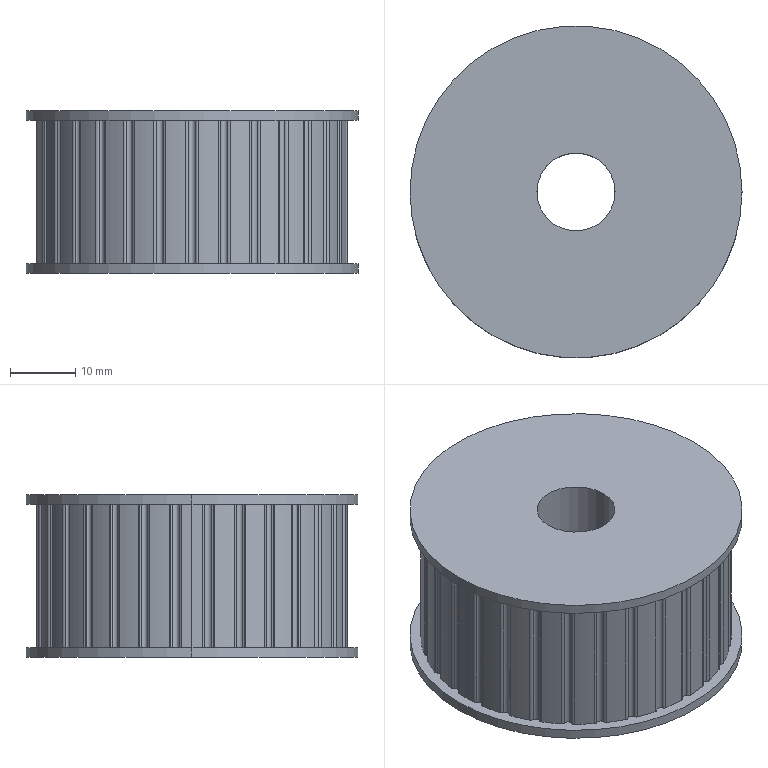Part | 1 solid | 151 faces | box 51 x 51 x 25 mm | volume 42334 mm3 | cylinder 147 | plane 4 | commonest cylinder face diameters 0.96 x70 1.14 x40 47.75 x31 51 x4 12 x2